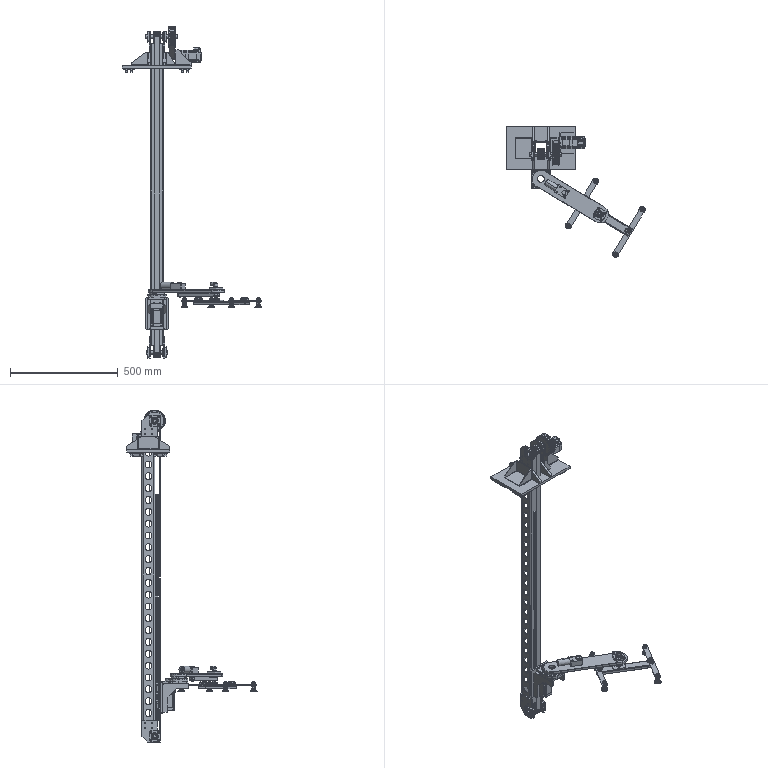Part | SolidWorks | 204 solids | 12111 faces | volume 4751526 mm3 | plane 5358 | cylinder 3679 | cone 1011 | spline 748 | torus 663 | sphere 652 | commonest cylinder face diameters 0.5 x336 6.55 x336 1.1 x332 1.459 x186 32 x164 6 x150